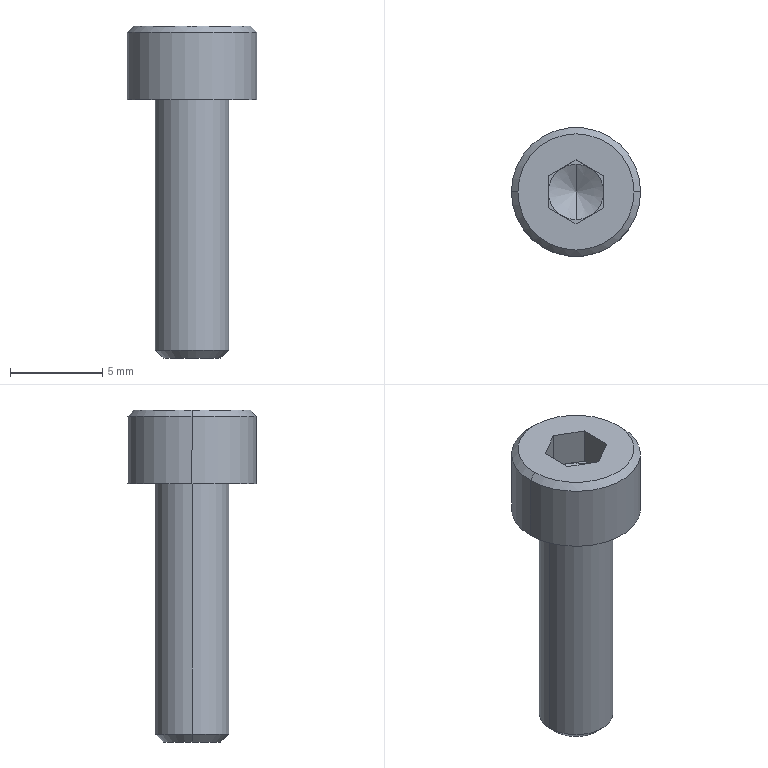Part | NX | features BREP 1 | 1 solid | 25 faces | box 7 x 7 x 18 mm | volume 309.86 mm3 | plane 15 | cone 6 | cylinder 4 | commonest cylinder face diameters 4 x2 7 x2
STEP:
#1=CARTESIAN_POINT('',(0.,-1.5,2.));
#2=VERTEX_POINT('',#1);
#3=CARTESIAN_POINT('',(0.,0.,1.134));
#4=VERTEX_POINT('',#3);
#5=CARTESIAN_POINT('',(0.,0.,1.134));
#6=DIRECTION('',(0.,-0.866,0.5));
#7=VECTOR('',#6,1000.);
#8=LINE('',#5,#7);
#9=EDGE_CURVE('',#2,#4,#8,.F.);
#10=ORIENTED_EDGE('',*,*,#9,.T.);
#11=CARTESIAN_POINT('',(0.,1.5,2.));
#12=VERTEX_POINT('',#11);
#13=CARTESIAN_POINT('',(0.,0.,1.134));
#14=DIRECTION('',(0.,0.866,0.5));
#15=VECTOR('',#14,1000.);
#16=LINE('',#13,#15);
#17=EDGE_CURVE('',#12,#4,#16,.F.);
#18=ORIENTED_EDGE('',*,*,#17,.F.);
#19=CARTESIAN_POINT('',(-0.75,1.299,2.));
#20=VERTEX_POINT('',#19);
#21=CARTESIAN_POINT('',(0.,0.,2.));
#22=DIRECTION('',(0.,0.,1.));
#23=DIRECTION('',(0.,-1.,0.));
#24=AXIS2_PLACEMENT_3D('',#21,#22,#23);
#25=CIRCLE('',#24,1.5);
#26=EDGE_CURVE('',#12,#20,#25,.T.);
#27=ORIENTED_EDGE('',*,*,#26,.T.);
#28=CARTESIAN_POINT('',(-1.5,0.,2.));
#29=VERTEX_POINT('',#28);
#30=CARTESIAN_POINT('',(0.,0.,2.));
#31=DIRECTION('',(0.,0.,1.));
#32=DIRECTION('',(0.,-1.,0.));
#33=AXIS2_PLACEMENT_3D('',#30,#31,#32);
#34=CIRCLE('',#33,1.5);
#35=EDGE_CURVE('',#20,#29,#34,.T.);
#36=ORIENTED_EDGE('',*,*,#35,.T.);
#37=CARTESIAN_POINT('',(-0.75,-1.299,2.));
#38=VERTEX_POINT('',#37);
#39=CARTESIAN_POINT('',(0.,0.,2.));
#40=DIRECTION('',(0.,0.,1.));
#41=DIRECTION('',(0.,-1.,0.));
#42=AXIS2_PLACEMENT_3D('',#39,#40,#41);
#43=CIRCLE('',#42,1.5);
#44=EDGE_CURVE('',#29,#38,#43,.T.);
#45=ORIENTED_EDGE('',*,*,#44,.T.);
#46=CARTESIAN_POINT('',(0.,0.,2.));
#47=DIRECTION('',(0.,0.,1.));
#48=DIRECTION('',(0.,-1.,0.));
#49=AXIS2_PLACEMENT_3D('',#46,#47,#48);
#50=CIRCLE('',#49,1.5);
#51=EDGE_CURVE('',#38,#2,#50,.T.);
#52=ORIENTED_EDGE('',*,*,#51,.T.);
#53=EDGE_LOOP('',(#10,#18,#27,#36,#45,#52));
#54=FACE_BOUND('',#53,.T.);
#55=CARTESIAN_POINT('',(0.,0.,1001.134));
#56=DIRECTION('',(0.,0.,1.));
#57=DIRECTION('',(0.,1.,0.));
#58=AXIS2_PLACEMENT_3D('',#55,#56,#57);
#59=CONICAL_SURFACE('',#58,1732.051,1.047);
#60=ADVANCED_FACE('',(#54),#59,.F.);
#61=CARTESIAN_POINT('',(3.5,0.,0.));
#62=VERTEX_POINT('',#61);
#63=CARTESIAN_POINT('',(-3.5,0.,0.));
#64=VERTEX_POINT('',#63);
#65=CARTESIAN_POINT('',(0.,0.,0.));
#66=DIRECTION('',(0.,0.,1.));
#67=DIRECTION('',(1.,0.,0.));
#68=AXIS2_PLACEMENT_3D('',#65,#66,#67);
#69=CIRCLE('',#68,3.5);
#70=EDGE_CURVE('',#62,#64,#69,.T.);
#71=ORIENTED_EDGE('',*,*,#70,.T.);
#72=CARTESIAN_POINT('',(-3.5,0.,3.65));
#73=VERTEX_POINT('',#72);
#74=CARTESIAN_POINT('',(-3.5,0.,0.));
#75=DIRECTION('',(0.,0.,1.));
#76=VECTOR('',#75,1000.);
#77=LINE('',#74,#76);
#78=EDGE_CURVE('',#64,#73,#77,.T.);
#79=ORIENTED_EDGE('',*,*,#78,.T.);
#80=CARTESIAN_POINT('',(3.5,0.,3.65));
#81=VERTEX_POINT('',#80);
#82=CARTESIAN_POINT('',(0.,0.,3.65));
#83=DIRECTION('',(0.,0.,1.));
#84=DIRECTION('',(1.,0.,0.));
#85=AXIS2_PLACEMENT_3D('',#82,#83,#84);
#86=CIRCLE('',#85,3.5);
#87=EDGE_CURVE('',#81,#73,#86,.T.);
#88=ORIENTED_EDGE('',*,*,#87,.F.);
#89=CARTESIAN_POINT('',(3.5,0.,0.));
#90=DIRECTION('',(0.,0.,1.));
#91=VECTOR('',#90,1000.);
#92=LINE('',#89,#91);
#93=EDGE_CURVE('',#62,#81,#92,.T.);
#94=ORIENTED_EDGE('',*,*,#93,.F.);
#95=EDGE_LOOP('',(#71,#79,#88,#94));
#96=FACE_BOUND('',#95,.T.);
#97=CARTESIAN_POINT('',(0.,0.,0.));
#98=DIRECTION('',(0.,0.,1.));
#99=DIRECTION('',(-1.,0.,0.));
#100=AXIS2_PLACEMENT_3D('',#97,#98,#99);
#101=CYLINDRICAL_SURFACE('',#100,3.5);
#102=ADVANCED_FACE('',(#96),#101,.T.);
#103=CARTESIAN_POINT('',(3.15,0.,4.));
#104=VERTEX_POINT('',#103);
#105=CARTESIAN_POINT('',(-3.15,0.,4.));
#106=VERTEX_POINT('',#105);
#107=CARTESIAN_POINT('',(0.,0.,4.));
#108=DIRECTION('',(0.,0.,1.));
#109=DIRECTION('',(1.,0.,0.));
#110=AXIS2_PLACEMENT_3D('',#107,#108,#109);
#111=CIRCLE('',#110,3.15);
#112=EDGE_CURVE('',#104,#106,#111,.T.);
#113=ORIENTED_EDGE('',*,*,#112,.F.);
#114=CARTESIAN_POINT('',(3.5,0.,3.65));
#115=DIRECTION('',(0.7071,0.,-0.7071));
#116=VECTOR('',#115,1000.);
#117=LINE('',#114,#116);
#118=EDGE_CURVE('',#81,#104,#117,.F.);
#119=ORIENTED_EDGE('',*,*,#118,.F.);
#120=ORIENTED_EDGE('',*,*,#87,.T.);
#121=CARTESIAN_POINT('',(-3.5,0.,3.65));
#122=DIRECTION('',(-0.7071,0.,-0.7071));
#123=VECTOR('',#122,1000.);
#124=LINE('',#121,#123);
#125=EDGE_CURVE('',#73,#106,#124,.F.);
#126=ORIENTED_EDGE('',*,*,#125,.T.);
#127=EDGE_LOOP('',(#113,#119,#120,#126));
#128=FACE_BOUND('',#127,.T.);
#129=CARTESIAN_POINT('',(0.,0.,3.65));
#130=DIRECTION('',(0.,0.,-1.));
#131=DIRECTION('',(1.,0.,0.));
#132=AXIS2_PLACEMENT_3D('',#129,#130,#131);
#133=CONICAL_SURFACE('',#132,3.5,0.7854);
#134=ADVANCED_FACE('',(#128),#133,.T.);
#135=CARTESIAN_POINT('',(1.571,0.,-14.));
#136=VERTEX_POINT('',#135);
#137=CARTESIAN_POINT('',(-1.571,0.,-14.));
#138=VERTEX_POINT('',#137);
#139=CARTESIAN_POINT('',(0.,0.,-14.));
#140=DIRECTION('',(0.,0.,1.));
#141=DIRECTION('',(1.,0.,0.));
#142=AXIS2_PLACEMENT_3D('',#139,#140,#141);
#143=CIRCLE('',#142,1.571);
#144=EDGE_CURVE('',#136,#138,#143,.T.);
#145=ORIENTED_EDGE('',*,*,#144,.T.);
#146=CARTESIAN_POINT('',(-2.,0.,-13.57));
#147=VERTEX_POINT('',#146);
#148=CARTESIAN_POINT('',(-1.571,0.,-14.));
#149=DIRECTION('',(-0.7071,0.,0.7071));
#150=VECTOR('',#149,1000.);
#151=LINE('',#148,#150);
#152=EDGE_CURVE('',#138,#147,#151,.T.);
#153=ORIENTED_EDGE('',*,*,#152,.T.);
#154=CARTESIAN_POINT('',(2.,0.,-13.57));
#155=VERTEX_POINT('',#154);
#156=CARTESIAN_POINT('',(0.,0.,-13.57));
#157=DIRECTION('',(0.,0.,1.));
#158=DIRECTION('',(1.,0.,0.));
#159=AXIS2_PLACEMENT_3D('',#156,#157,#158);
#160=CIRCLE('',#159,2.);
#161=EDGE_CURVE('',#155,#147,#160,.T.);
#162=ORIENTED_EDGE('',*,*,#161,.F.);
#163=CARTESIAN_POINT('',(1.571,0.,-14.));
#164=DIRECTION('',(0.7071,0.,0.7071));
#165=VECTOR('',#164,1000.);
#166=LINE('',#163,#165);
#167=EDGE_CURVE('',#136,#155,#166,.T.);
#168=ORIENTED_EDGE('',*,*,#167,.F.);
#169=EDGE_LOOP('',(#145,#153,#162,#168));
#170=FACE_BOUND('',#169,.T.);
#171=CARTESIAN_POINT('',(0.,0.,-14.));
#172=DIRECTION('',(0.,0.,1.));
#173=DIRECTION('',(-1.,0.,0.));
#174=AXIS2_PLACEMENT_3D('',#171,#172,#173);
#175=CONICAL_SURFACE('',#174,1.571,0.7854);
#176=ADVANCED_FACE('',(#170),#175,.T.);
#177=ORIENTED_EDGE('',*,*,#161,.T.);
#178=CARTESIAN_POINT('',(-2.,0.,0.));
#179=VERTEX_POINT('',#178);
#180=CARTESIAN_POINT('',(-2.,0.,-14.));
#181=DIRECTION('',(0.,0.,1.));
#182=VECTOR('',#181,1000.);
#183=LINE('',#180,#182);
#184=EDGE_CURVE('',#147,#179,#183,.T.);
#185=ORIENTED_EDGE('',*,*,#184,.T.);
#186=CARTESIAN_POINT('',(2.,0.,0.));
#187=VERTEX_POINT('',#186);
#188=CARTESIAN_POINT('',(0.,0.,0.));
#189=DIRECTION('',(0.,0.,1.));
#190=DIRECTION('',(1.,0.,0.));
#191=AXIS2_PLACEMENT_3D('',#188,#189,#190);
#192=CIRCLE('',#191,2.);
#193=EDGE_CURVE('',#187,#179,#192,.T.);
#194=ORIENTED_EDGE('',*,*,#193,.F.);
#195=CARTESIAN_POINT('',(2.,0.,-14.));
#196=DIRECTION('',(0.,0.,1.));
#197=VECTOR('',#196,1000.);
#198=LINE('',#195,#197);
#199=EDGE_CURVE('',#155,#187,#198,.T.);
#200=ORIENTED_EDGE('',*,*,#199,.F.);
#201=EDGE_LOOP('',(#177,#185,#194,#200));
#202=FACE_BOUND('',#201,.T.);
#203=CARTESIAN_POINT('',(0.,0.,-14.));
#204=DIRECTION('',(0.,0.,1.));
#205=DIRECTION('',(-1.,0.,0.));
#206=AXIS2_PLACEMENT_3D('',#203,#204,#205);
#207=CYLINDRICAL_SURFACE('',#206,2.);
#208=ADVANCED_FACE('',(#202),#207,.T.);
#209=CARTESIAN_POINT('',(0.75,-1.299,2.));
#210=VERTEX_POINT('',#209);
#211=CARTESIAN_POINT('',(1.5,0.,2.));
#212=VERTEX_POINT('',#211);
#213=CARTESIAN_POINT('',(0.,0.,2.));
#214=DIRECTION('',(0.,0.,1.));
#215=DIRECTION('',(0.,-1.,0.));
#216=AXIS2_PLACEMENT_3D('',#213,#214,#215);
#217=CIRCLE('',#216,1.5);
#218=EDGE_CURVE('',#210,#212,#217,.T.);
#219=ORIENTED_EDGE('',*,*,#218,.F.);
#220=CARTESIAN_POINT('',(1.5,-0.866,2.));
#221=VERTEX_POINT('',#220);
#222=CARTESIAN_POINT('',(0.,-1.732,2.));
#223=DIRECTION('',(0.866,0.5,0.));
#224=VECTOR('',#223,1000.);
#225=LINE('',#222,#224);
#226=EDGE_CURVE('',#210,#221,#225,.T.);
#227=ORIENTED_EDGE('',*,*,#226,.T.);
#228=CARTESIAN_POINT('',(1.5,-0.866,2.));
#229=DIRECTION('',(0.,1.,0.));
#230=VECTOR('',#229,1000.);
#231=LINE('',#228,#230);
#232=EDGE_CURVE('',#221,#212,#231,.T.);
#233=ORIENTED_EDGE('',*,*,#232,.T.);
#234=EDGE_LOOP('',(#219,#227,#233));
#235=FACE_BOUND('',#234,.T.);
#236=CARTESIAN_POINT('',(0.,0.,2.));
#237=DIRECTION('',(0.,0.,1.));
#238=DIRECTION('',(-1.,0.,0.));
#239=AXIS2_PLACEMENT_3D('',#236,#237,#238);
#240=PLANE('',#239);
#241=ADVANCED_FACE('',(#235),#240,.T.);
#242=CARTESIAN_POINT('',(0.75,1.299,2.));
#243=VERTEX_POINT('',#242);
#244=CARTESIAN_POINT('',(0.,0.,2.));
#245=DIRECTION('',(0.,0.,1.));
#246=DIRECTION('',(0.,-1.,0.));
#247=AXIS2_PLACEMENT_3D('',#244,#245,#246);
#248=CIRCLE('',#247,1.5);
#249=EDGE_CURVE('',#212,#243,#248,.T.);
#250=ORIENTED_EDGE('',*,*,#249,.F.);
#251=CARTESIAN_POINT('',(1.5,0.866,2.));
#252=VERTEX_POINT('',#251);
#253=CARTESIAN_POINT('',(1.5,-0.866,2.));
#254=DIRECTION('',(0.,1.,0.));
#255=VECTOR('',#254,1000.);
#256=LINE('',#253,#255);
#257=EDGE_CURVE('',#212,#252,#256,.T.);
#258=ORIENTED_EDGE('',*,*,#257,.T.);
#259=CARTESIAN_POINT('',(1.5,0.866,2.));
#260=DIRECTION('',(-0.866,0.5,0.));
#261=VECTOR('',#260,1000.);
#262=LINE('',#259,#261);
#263=EDGE_CURVE('',#252,#243,#262,.T.);
#264=ORIENTED_EDGE('',*,*,#263,.T.);
#265=EDGE_LOOP('',(#250,#258,#264));
#266=FACE_BOUND('',#265,.T.);
#267=CARTESIAN_POINT('',(0.,0.,2.));
#268=DIRECTION('',(0.,0.,1.));
#269=DIRECTION('',(-1.,0.,0.));
#270=AXIS2_PLACEMENT_3D('',#267,#268,#269);
#271=PLANE('',#270);
#272=ADVANCED_FACE('',(#266),#271,.T.);
#273=CARTESIAN_POINT('',(0.,0.,2.));
#274=DIRECTION('',(0.,0.,1.));
#275=DIRECTION('',(0.,-1.,0.));
#276=AXIS2_PLACEMENT_3D('',#273,#274,#275);
#277=CIRCLE('',#276,1.5);
#278=EDGE_CURVE('',#243,#12,#277,.T.);
#279=ORIENTED_EDGE('',*,*,#278,.F.);
#280=CARTESIAN_POINT('',(0.,1.732,2.));
#281=VERTEX_POINT('',#280);
#282=CARTESIAN_POINT('',(1.5,0.866,2.));
#283=DIRECTION('',(-0.866,0.5,0.));
#284=VECTOR('',#283,1000.);
#285=LINE('',#282,#284);
#286=EDGE_CURVE('',#243,#281,#285,.T.);
#287=ORIENTED_EDGE('',*,*,#286,.T.);
#288=CARTESIAN_POINT('',(0.,1.732,2.));
#289=DIRECTION('',(-0.866,-0.5,0.));
#290=VECTOR('',#289,1000.);
#291=LINE('',#288,#290);
#292=EDGE_CURVE('',#281,#20,#291,.T.);
#293=ORIENTED_EDGE('',*,*,#292,.T.);
#294=ORIENTED_EDGE('',*,*,#26,.F.);
#295=EDGE_LOOP('',(#279,#287,#293,#294));
#296=FACE_BOUND('',#295,.T.);
#297=CARTESIAN_POINT('',(0.,0.,2.));
#298=DIRECTION('',(0.,0.,1.));
#299=DIRECTION('',(-1.,0.,0.));
#300=AXIS2_PLACEMENT_3D('',#297,#298,#299);
#301=PLANE('',#300);
#302=ADVANCED_FACE('',(#296),#301,.T.);
#303=ORIENTED_EDGE('',*,*,#35,.F.);
#304=CARTESIAN_POINT('',(-1.5,0.866,2.));
#305=VERTEX_POINT('',#304);
#306=CARTESIAN_POINT('',(0.,1.732,2.));
#307=DIRECTION('',(-0.866,-0.5,0.));
#308=VECTOR('',#307,1000.);
#309=LINE('',#306,#308);
#310=EDGE_CURVE('',#20,#305,#309,.T.);
#311=ORIENTED_EDGE('',*,*,#310,.T.);
#312=CARTESIAN_POINT('',(-1.5,0.866,2.));
#313=DIRECTION('',(0.,-1.,0.));
#314=VECTOR('',#313,1000.);
#315=LINE('',#312,#314);
#316=EDGE_CURVE('',#305,#29,#315,.T.);
#317=ORIENTED_EDGE('',*,*,#316,.T.);
#318=EDGE_LOOP('',(#303,#311,#317));
#319=FACE_BOUND('',#318,.T.);
#320=CARTESIAN_POINT('',(0.,0.,2.));
#321=DIRECTION('',(0.,0.,1.));
#322=DIRECTION('',(-1.,0.,0.));
#323=AXIS2_PLACEMENT_3D('',#320,#321,#322);
#324=PLANE('',#323);
#325=ADVANCED_FACE('',(#319),#324,.T.);
#326=ORIENTED_EDGE('',*,*,#44,.F.);
#327=CARTESIAN_POINT('',(-1.5,-0.866,2.));
#328=VERTEX_POINT('',#327);
#329=CARTESIAN_POINT('',(-1.5,0.866,2.));
#330=DIRECTION('',(0.,-1.,0.));
#331=VECTOR('',#330,1000.);
#332=LINE('',#329,#331);
#333=EDGE_CURVE('',#29,#328,#332,.T.);
#334=ORIENTED_EDGE('',*,*,#333,.T.);
#335=CARTESIAN_POINT('',(-1.5,-0.866,2.));
#336=DIRECTION('',(0.866,-0.5,0.));
#337=VECTOR('',#336,1000.);
#338=LINE('',#335,#337);
#339=EDGE_CURVE('',#328,#38,#338,.T.);
#340=ORIENTED_EDGE('',*,*,#339,.T.);
#341=EDGE_LOOP('',(#326,#334,#340));
#342=FACE_BOUND('',#341,.T.);
#343=CARTESIAN_POINT('',(0.,0.,2.));
#344=DIRECTION('',(0.,0.,1.));
#345=DIRECTION('',(-1.,0.,0.));
#346=AXIS2_PLACEMENT_3D('',#343,#344,#345);
#347=PLANE('',#346);
#348=ADVANCED_FACE('',(#342),#347,.T.);
#349=ORIENTED_EDGE('',*,*,#184,.F.);
#350=CARTESIAN_POINT('',(0.,0.,-13.57));
#351=DIRECTION('',(0.,0.,1.));
#352=DIRECTION('',(1.,0.,0.));
#353=AXIS2_PLACEMENT_3D('',#350,#351,#352);
#354=CIRCLE('',#353,2.);
#355=EDGE_CURVE('',#147,#155,#354,.T.);
#356=ORIENTED_EDGE('',*,*,#355,.T.);
#357=ORIENTED_EDGE('',*,*,#199,.T.);
#358=CARTESIAN_POINT('',(0.,0.,0.));
#359=DIRECTION('',(0.,0.,1.));
#360=DIRECTION('',(1.,0.,0.));
#361=AXIS2_PLACEMENT_3D('',#358,#359,#360);
#362=CIRCLE('',#361,2.);
#363=EDGE_CURVE('',#179,#187,#362,.T.);
#364=ORIENTED_EDGE('',*,*,#363,.F.);
#365=EDGE_LOOP('',(#349,#356,#357,#364));
#366=FACE_BOUND('',#365,.T.);
#367=CARTESIAN_POINT('',(0.,0.,-14.));
#368=DIRECTION('',(0.,0.,1.));
#369=DIRECTION('',(-1.,0.,0.));
#370=AXIS2_PLACEMENT_3D('',#367,#368,#369);
#371=CYLINDRICAL_SURFACE('',#370,2.);
#372=ADVANCED_FACE('',(#366),#371,.T.);
#373=ORIENTED_EDGE('',*,*,#152,.F.);
#374=CARTESIAN_POINT('',(0.,0.,-14.));
#375=DIRECTION('',(0.,0.,1.));
#376=DIRECTION('',(1.,0.,0.));
#377=AXIS2_PLACEMENT_3D('',#374,#375,#376);
#378=CIRCLE('',#377,1.571);
#379=EDGE_CURVE('',#138,#136,#378,.T.);
#380=ORIENTED_EDGE('',*,*,#379,.T.);
#381=ORIENTED_EDGE('',*,*,#167,.T.);
#382=ORIENTED_EDGE('',*,*,#355,.F.);
#383=EDGE_LOOP('',(#373,#380,#381,#382));
#384=FACE_BOUND('',#383,.T.);
#385=CARTESIAN_POINT('',(0.,0.,-14.));
#386=DIRECTION('',(0.,0.,1.));
#387=DIRECTION('',(-1.,0.,0.));
#388=AXIS2_PLACEMENT_3D('',#385,#386,#387);
#389=CONICAL_SURFACE('',#388,1.571,0.7854);
#390=ADVANCED_FACE('',(#384),#389,.T.);
#391=ORIENTED_EDGE('',*,*,#144,.F.);
#392=ORIENTED_EDGE('',*,*,#379,.F.);
#393=EDGE_LOOP('',(#391,#392));
#394=FACE_BOUND('',#393,.T.);
#395=CARTESIAN_POINT('',(0.,1.571,-14.));
#396=DIRECTION('',(0.,0.,1.));
#397=DIRECTION('',(-1.,0.,0.));
#398=AXIS2_PLACEMENT_3D('',#395,#396,#397);
#399=PLANE('',#398);
#400=ADVANCED_FACE('',(#394),#399,.F.);
#401=CARTESIAN_POINT('',(0.,-1.732,4.));
#402=VERTEX_POINT('',#401);
#403=CARTESIAN_POINT('',(1.5,-0.866,4.));
#404=VERTEX_POINT('',#403);
#405=CARTESIAN_POINT('',(0.,-1.732,4.));
#406=DIRECTION('',(0.866,0.5,0.));
#407=VECTOR('',#406,1000.);
#408=LINE('',#405,#407);
#409=EDGE_CURVE('',#402,#404,#408,.T.);
#410=ORIENTED_EDGE('',*,*,#409,.F.);
#411=CARTESIAN_POINT('',(-1.5,-0.866,4.));
#412=VERTEX_POINT('',#411);
#413=CARTESIAN_POINT('',(-1.5,-0.866,4.));
#414=DIRECTION('',(0.866,-0.5,0.));
#415=VECTOR('',#414,1000.);
#416=LINE('',#413,#415);
#417=EDGE_CURVE('',#412,#402,#416,.T.);
#418=ORIENTED_EDGE('',*,*,#417,.F.);
#419=CARTESIAN_POINT('',(-1.5,0.866,4.));
#420=VERTEX_POINT('',#419);
#421=CARTESIAN_POINT('',(-1.5,0.866,4.));
#422=DIRECTION('',(0.,-1.,0.));
#423=VECTOR('',#422,1000.);
#424=LINE('',#421,#423);
#425=EDGE_CURVE('',#420,#412,#424,.T.);
#426=ORIENTED_EDGE('',*,*,#425,.F.);
#427=CARTESIAN_POINT('',(0.,1.732,4.));
#428=VERTEX_POINT('',#427);
#429=CARTESIAN_POINT('',(0.,1.732,4.));
#430=DIRECTION('',(-0.866,-0.5,0.));
#431=VECTOR('',#430,1000.);
#432=LINE('',#429,#431);
#433=EDGE_CURVE('',#428,#420,#432,.T.);
#434=ORIENTED_EDGE('',*,*,#433,.F.);
#435=CARTESIAN_POINT('',(1.5,0.866,4.));
#436=VERTEX_POINT('',#435);
#437=CARTESIAN_POINT('',(1.5,0.866,4.));
#438=DIRECTION('',(-0.866,0.5,0.));
#439=VECTOR('',#438,1000.);
#440=LINE('',#437,#439);
#441=EDGE_CURVE('',#436,#428,#440,.T.);
#442=ORIENTED_EDGE('',*,*,#441,.F.);
#443=CARTESIAN_POINT('',(1.5,-0.866,4.));
#444=DIRECTION('',(0.,1.,0.));
#445=VECTOR('',#444,1000.);
#446=LINE('',#443,#445);
#447=EDGE_CURVE('',#404,#436,#446,.T.);
#448=ORIENTED_EDGE('',*,*,#447,.F.);
#449=EDGE_LOOP('',(#410,#418,#426,#434,#442,#448));
#450=FACE_BOUND('',#449,.T.);
#451=CARTESIAN_POINT('',(0.,0.,4.));
#452=DIRECTION('',(0.,0.,1.));
#453=DIRECTION('',(1.,0.,0.));
#454=AXIS2_PLACEMENT_3D('',#451,#452,#453);
#455=CIRCLE('',#454,3.15);
#456=EDGE_CURVE('',#106,#104,#455,.T.);
#457=ORIENTED_EDGE('',*,*,#456,.T.);
#458=ORIENTED_EDGE('',*,*,#112,.T.);
#459=EDGE_LOOP('',(#457,#458));
#460=FACE_BOUND('',#459,.T.);
#461=CARTESIAN_POINT('',(0.,0.,4.));
#462=DIRECTION('',(0.,0.,-1.));
#463=DIRECTION('',(1.,0.,0.));
#464=AXIS2_PLACEMENT_3D('',#461,#462,#463);
#465=PLANE('',#464);
#466=ADVANCED_FACE('',(#450,#460),#465,.F.);
#467=ORIENTED_EDGE('',*,*,#118,.T.);
#468=ORIENTED_EDGE('',*,*,#456,.F.);
#469=ORIENTED_EDGE('',*,*,#125,.F.);
#470=CARTESIAN_POINT('',(0.,0.,3.65));
#471=DIRECTION('',(0.,0.,1.));
#472=DIRECTION('',(1.,0.,0.));
#473=AXIS2_PLACEMENT_3D('',#470,#471,#472);
#474=CIRCLE('',#473,3.5);
#475=EDGE_CURVE('',#73,#81,#474,.T.);
#476=ORIENTED_EDGE('',*,*,#475,.T.);
#477=EDGE_LOOP('',(#467,#468,#469,#476));
#478=FACE_BOUND('',#477,.T.);
#479=CARTESIAN_POINT('',(0.,0.,3.65));
#480=DIRECTION('',(0.,0.,-1.));
#481=DIRECTION('',(1.,0.,0.));
#482=AXIS2_PLACEMENT_3D('',#479,#480,#481);
#483=CONICAL_SURFACE('',#482,3.5,0.7854);
#484=ADVANCED_FACE('',(#478),#483,.T.);
#485=ORIENTED_EDGE('',*,*,#78,.F.);
#486=CARTESIAN_POINT('',(0.,0.,0.));
#487=DIRECTION('',(0.,0.,1.));
#488=DIRECTION('',(1.,0.,0.));
#489=AXIS2_PLACEMENT_3D('',#486,#487,#488);
#490=CIRCLE('',#489,3.5);
#491=EDGE_CURVE('',#64,#62,#490,.T.);
#492=ORIENTED_EDGE('',*,*,#491,.T.);
#493=ORIENTED_EDGE('',*,*,#93,.T.);
#494=ORIENTED_EDGE('',*,*,#475,.F.);
#495=EDGE_LOOP('',(#485,#492,#493,#494));
#496=FACE_BOUND('',#495,.T.);
#497=CARTESIAN_POINT('',(0.,0.,0.));
#498=DIRECTION('',(0.,0.,1.));
#499=DIRECTION('',(-1.,0.,0.));
#500=AXIS2_PLACEMENT_3D('',#497,#498,#499);
#501=CYLINDRICAL_SURFACE('',#500,3.5);
#502=ADVANCED_FACE('',(#496),#501,.T.);
#503=ORIENTED_EDGE('',*,*,#193,.T.);
#504=ORIENTED_EDGE('',*,*,#363,.T.);
#505=EDGE_LOOP('',(#503,#504));
#506=FACE_BOUND('',#505,.T.);
#507=ORIENTED_EDGE('',*,*,#70,.F.);
#508=ORIENTED_EDGE('',*,*,#491,.F.);
#509=EDGE_LOOP('',(#507,#508));
#510=FACE_BOUND('',#509,.T.);
#511=CARTESIAN_POINT('',(0.,3.5,0.));
#512=DIRECTION('',(0.,0.,1.));
#513=DIRECTION('',(-1.,0.,0.));
#514=AXIS2_PLACEMENT_3D('',#511,#512,#513);
#515=PLANE('',#514);
#516=ADVANCED_FACE('',(#506,#510),#515,.F.);
#517=ORIENTED_EDGE('',*,*,#417,.T.);
#518=CARTESIAN_POINT('',(0.,-1.732,2.));
#519=VERTEX_POINT('',#518);
#520=CARTESIAN_POINT('',(0.,-1.732,2.));
#521=DIRECTION('',(0.,0.,1.));
#522=VECTOR('',#521,1000.);
#523=LINE('',#520,#522);
#524=EDGE_CURVE('',#519,#402,#523,.T.);
#525=ORIENTED_EDGE('',*,*,#524,.F.);
#526=CARTESIAN_POINT('',(-1.5,-0.866,2.));
#527=DIRECTION('',(0.866,-0.5,0.));
#528=VECTOR('',#527,1000.);
#529=LINE('',#526,#528);
#530=EDGE_CURVE('',#38,#519,#529,.T.);
#531=ORIENTED_EDGE('',*,*,#530,.F.);
#532=ORIENTED_EDGE('',*,*,#339,.F.);
#533=CARTESIAN_POINT('',(-1.5,-0.866,2.));
#534=DIRECTION('',(0.,0.,1.));
#535=VECTOR('',#534,1000.);
#536=LINE('',#533,#535);
#537=EDGE_CURVE('',#328,#412,#536,.T.);
#538=ORIENTED_EDGE('',*,*,#537,.T.);
#539=EDGE_LOOP('',(#517,#525,#531,#532,#538));
#540=FACE_BOUND('',#539,.T.);
#541=CARTESIAN_POINT('',(-1.5,-0.866,2.));
#542=DIRECTION('',(-0.5,-0.866,0.));
#543=DIRECTION('',(-0.866,0.5,0.));
#544=AXIS2_PLACEMENT_3D('',#541,#542,#543);
#545=PLANE('',#544);
#546=ADVANCED_FACE('',(#540),#545,.F.);
#547=ORIENTED_EDGE('',*,*,#425,.T.);
#548=ORIENTED_EDGE('',*,*,#537,.F.);
#549=ORIENTED_EDGE('',*,*,#333,.F.);
#550=ORIENTED_EDGE('',*,*,#316,.F.);
#551=CARTESIAN_POINT('',(-1.5,0.866,2.));
#552=DIRECTION('',(0.,0.,1.));
#553=VECTOR('',#552,1000.);
#554=LINE('',#551,#553);
#555=EDGE_CURVE('',#305,#420,#554,.T.);
#556=ORIENTED_EDGE('',*,*,#555,.T.);
#557=EDGE_LOOP('',(#547,#548,#549,#550,#556));
#558=FACE_BOUND('',#557,.T.);
#559=CARTESIAN_POINT('',(-1.5,0.866,2.));
#560=DIRECTION('',(-1.,0.,0.));
#561=DIRECTION('',(0.,0.,-1.));
#562=AXIS2_PLACEMENT_3D('',#559,#560,#561);
#563=PLANE('',#562);
#564=ADVANCED_FACE('',(#558),#563,.F.);
#565=ORIENTED_EDGE('',*,*,#433,.T.);
#566=ORIENTED_EDGE('',*,*,#555,.F.);
#567=ORIENTED_EDGE('',*,*,#310,.F.);
#568=ORIENTED_EDGE('',*,*,#292,.F.);
#569=CARTESIAN_POINT('',(0.,1.732,2.));
#570=DIRECTION('',(0.,0.,1.));
#571=VECTOR('',#570,1000.);
#572=LINE('',#569,#571);
#573=EDGE_CURVE('',#281,#428,#572,.T.);
#574=ORIENTED_EDGE('',*,*,#573,.T.);
#575=EDGE_LOOP('',(#565,#566,#567,#568,#574));
#576=FACE_BOUND('',#575,.T.);
#577=CARTESIAN_POINT('',(0.,1.732,2.));
#578=DIRECTION('',(-0.5,0.866,0.));
#579=DIRECTION('',(0.866,0.5,0.));
#580=AXIS2_PLACEMENT_3D('',#577,#578,#579);
#581=PLANE('',#580);
#582=ADVANCED_FACE('',(#576),#581,.F.);
#583=ORIENTED_EDGE('',*,*,#441,.T.);
#584=ORIENTED_EDGE('',*,*,#573,.F.);
#585=ORIENTED_EDGE('',*,*,#286,.F.);
#586=ORIENTED_EDGE('',*,*,#263,.F.);
#587=CARTESIAN_POINT('',(1.5,0.866,2.));
#588=DIRECTION('',(0.,0.,1.));
#589=VECTOR('',#588,1000.);
#590=LINE('',#587,#589);
#591=EDGE_CURVE('',#252,#436,#590,.T.);
#592=ORIENTED_EDGE('',*,*,#591,.T.);
#593=EDGE_LOOP('',(#583,#584,#585,#586,#592));
#594=FACE_BOUND('',#593,.T.);
#595=CARTESIAN_POINT('',(1.5,0.866,2.));
#596=DIRECTION('',(0.5,0.866,0.));
#597=DIRECTION('',(0.866,-0.5,0.));
#598=AXIS2_PLACEMENT_3D('',#595,#596,#597);
#599=PLANE('',#598);
#600=ADVANCED_FACE('',(#594),#599,.F.);
#601=ORIENTED_EDGE('',*,*,#447,.T.);
#602=ORIENTED_EDGE('',*,*,#591,.F.);
#603=ORIENTED_EDGE('',*,*,#257,.F.);
#604=ORIENTED_EDGE('',*,*,#232,.F.);
#605=CARTESIAN_POINT('',(1.5,-0.866,2.));
#606=DIRECTION('',(0.,0.,1.));
#607=VECTOR('',#606,1000.);
#608=LINE('',#605,#607);
#609=EDGE_CURVE('',#221,#404,#608,.T.);
#610=ORIENTED_EDGE('',*,*,#609,.T.);
#611=EDGE_LOOP('',(#601,#602,#603,#604,#610));
#612=FACE_BOUND('',#611,.T.);
#613=CARTESIAN_POINT('',(1.5,-0.866,2.));
#614=DIRECTION('',(1.,0.,0.));
#615=DIRECTION('',(0.,0.,1.));
#616=AXIS2_PLACEMENT_3D('',#613,#614,#615);
#617=PLANE('',#616);
#618=ADVANCED_FACE('',(#612),#617,.F.);
#619=ORIENTED_EDGE('',*,*,#409,.T.);
#620=ORIENTED_EDGE('',*,*,#609,.F.);
#621=ORIENTED_EDGE('',*,*,#226,.F.);
#622=CARTESIAN_POINT('',(0.,-1.732,2.));
#623=DIRECTION('',(0.866,0.5,0.));
#624=VECTOR('',#623,1000.);
#625=LINE('',#622,#624);
#626=EDGE_CURVE('',#519,#210,#625,.T.);
#627=ORIENTED_EDGE('',*,*,#626,.F.);
#628=ORIENTED_EDGE('',*,*,#524,.T.);
#629=EDGE_LOOP('',(#619,#620,#621,#627,#628));
#630=FACE_BOUND('',#629,.T.);
#631=CARTESIAN_POINT('',(0.,-1.732,2.));
#632=DIRECTION('',(0.5,-0.866,0.));
#633=DIRECTION('',(-0.866,-0.5,0.));
#634=AXIS2_PLACEMENT_3D('',#631,#632,#633);
#635=PLANE('',#634);
#636=ADVANCED_FACE('',(#630),#635,.F.);
#637=ORIENTED_EDGE('',*,*,#51,.F.);
#638=ORIENTED_EDGE('',*,*,#530,.T.);
#639=ORIENTED_EDGE('',*,*,#626,.T.);
#640=CARTESIAN_POINT('',(0.,0.,2.));
#641=DIRECTION('',(0.,0.,1.));
#642=DIRECTION('',(0.,-1.,0.));
#643=AXIS2_PLACEMENT_3D('',#640,#641,#642);
#644=CIRCLE('',#643,1.5);
#645=EDGE_CURVE('',#2,#210,#644,.T.);
#646=ORIENTED_EDGE('',*,*,#645,.F.);
#647=EDGE_LOOP('',(#637,#638,#639,#646));
#648=FACE_BOUND('',#647,.T.);
#649=CARTESIAN_POINT('',(0.,0.,2.));
#650=DIRECTION('',(0.,0.,1.));
#651=DIRECTION('',(-1.,0.,0.));
#652=AXIS2_PLACEMENT_3D('',#649,#650,#651);
#653=PLANE('',#652);
#654=ADVANCED_FACE('',(#648),#653,.T.);
#655=ORIENTED_EDGE('',*,*,#17,.T.);
#656=ORIENTED_EDGE('',*,*,#9,.F.);
#657=ORIENTED_EDGE('',*,*,#645,.T.);
#658=ORIENTED_EDGE('',*,*,#218,.T.);
#659=ORIENTED_EDGE('',*,*,#249,.T.);
#660=ORIENTED_EDGE('',*,*,#278,.T.);
#661=EDGE_LOOP('',(#655,#656,#657,#658,#659,#660));
#662=FACE_BOUND('',#661,.T.);
#663=CARTESIAN_POINT('',(0.,0.,1001.134));
#664=DIRECTION('',(0.,0.,1.));
#665=DIRECTION('',(0.,1.,0.));
#666=AXIS2_PLACEMENT_3D('',#663,#664,#665);
#667=CONICAL_SURFACE('',#666,1732.051,1.047);
#668=ADVANCED_FACE('',(#662),#667,.F.);
#669=CLOSED_SHELL('',(#60,#102,#134,#176,#208,#241,#272,#302,#325,#348,#372,#390,#400,#466,#484,#502,#516,#546,#564,#582,#600,#618,#636,#654,#668));
#670=MANIFOLD_SOLID_BREP('',#669);
#671=(LENGTH_UNIT()NAMED_UNIT(*)SI_UNIT(.MILLI.,.METRE.));
#672=UNCERTAINTY_MEASURE_WITH_UNIT(LENGTH_MEASURE(0.00001),#671,'','');
#673=(NAMED_UNIT(*)PLANE_ANGLE_UNIT()SI_UNIT($,.RADIAN.));
#674=(NAMED_UNIT(*)SI_UNIT($,.STERADIAN.)SOLID_ANGLE_UNIT());
#675=(GEOMETRIC_REPRESENTATION_CONTEXT(3)GLOBAL_UNCERTAINTY_ASSIGNED_CONTEXT((#672))GLOBAL_UNIT_ASSIGNED_CONTEXT((#671,#673,#674))REPRESENTATION_CONTEXT('',''));
#676=ADVANCED_BREP_SHAPE_REPRESENTATION('',(#670),#675);